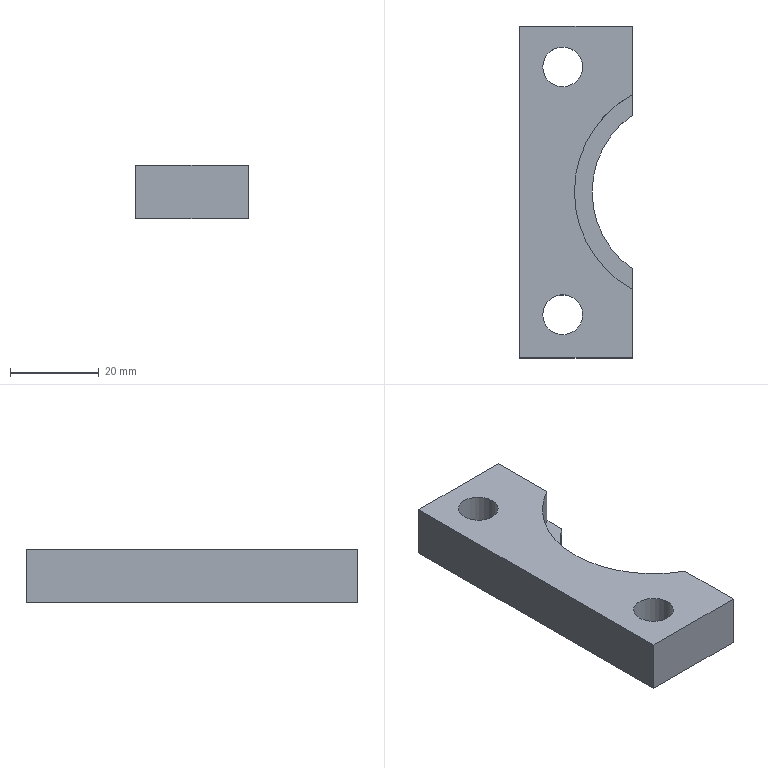Part | NX | features solid 2 | 1 solid | 12 faces | box 25.5 x 75 x 12 mm | volume 17248 mm3 | plane 8 | cylinder 4 | commonest cylinder face diameters 9 x2 42.2 x1 50.2 x1
STEP:
#1=CARTESIAN_POINT('',(697.5,172.5,250.));
#2=VERTEX_POINT('',#1);
#3=CARTESIAN_POINT('',(697.5,247.5,250.));
#4=VERTEX_POINT('',#3);
#5=CARTESIAN_POINT('',(697.5,172.5,250.));
#6=DIRECTION('',(0.,1.,0.));
#7=VECTOR('',#6,1000.);
#8=LINE('',#5,#7);
#9=EDGE_CURVE('',#2,#4,#8,.T.);
#10=ORIENTED_EDGE('',*,*,#9,.T.);
#11=CARTESIAN_POINT('',(697.5,247.5,238.));
#12=VERTEX_POINT('',#11);
#13=CARTESIAN_POINT('',(697.5,247.5,242.));
#14=DIRECTION('',(0.,0.,1.));
#15=VECTOR('',#14,1000.);
#16=LINE('',#13,#15);
#17=EDGE_CURVE('',#12,#4,#16,.T.);
#18=ORIENTED_EDGE('',*,*,#17,.F.);
#19=CARTESIAN_POINT('',(697.5,172.5,238.));
#20=VERTEX_POINT('',#19);
#21=CARTESIAN_POINT('',(697.5,172.5,238.));
#22=DIRECTION('',(0.,1.,0.));
#23=VECTOR('',#22,1000.);
#24=LINE('',#21,#23);
#25=EDGE_CURVE('',#20,#12,#24,.T.);
#26=ORIENTED_EDGE('',*,*,#25,.F.);
#27=CARTESIAN_POINT('',(697.5,172.5,242.));
#28=DIRECTION('',(0.,0.,1.));
#29=VECTOR('',#28,1000.);
#30=LINE('',#27,#29);
#31=EDGE_CURVE('',#20,#2,#30,.T.);
#32=ORIENTED_EDGE('',*,*,#31,.T.);
#33=EDGE_LOOP('',(#10,#18,#26,#32));
#34=FACE_BOUND('',#33,.T.);
#35=CARTESIAN_POINT('',(697.5,172.5,242.));
#36=DIRECTION('',(1.,0.,0.));
#37=DIRECTION('',(0.,0.,-1.));
#38=AXIS2_PLACEMENT_3D('',#35,#36,#37);
#39=PLANE('',#38);
#40=ADVANCED_FACE('',(#34),#39,.F.);
#41=CARTESIAN_POINT('',(723.,172.5,250.));
#42=VERTEX_POINT('',#41);
#43=CARTESIAN_POINT('',(723.,172.5,250.));
#44=DIRECTION('',(-1.,0.,0.));
#45=VECTOR('',#44,1000.);
#46=LINE('',#43,#45);
#47=EDGE_CURVE('',#42,#2,#46,.T.);
#48=ORIENTED_EDGE('',*,*,#47,.T.);
#49=ORIENTED_EDGE('',*,*,#31,.F.);
#50=CARTESIAN_POINT('',(723.,172.5,238.));
#51=VERTEX_POINT('',#50);
#52=CARTESIAN_POINT('',(723.,172.5,238.));
#53=DIRECTION('',(-1.,0.,0.));
#54=VECTOR('',#53,1000.);
#55=LINE('',#52,#54);
#56=EDGE_CURVE('',#51,#20,#55,.T.);
#57=ORIENTED_EDGE('',*,*,#56,.F.);
#58=CARTESIAN_POINT('',(723.,172.5,242.));
#59=DIRECTION('',(0.,0.,1.));
#60=VECTOR('',#59,1000.);
#61=LINE('',#58,#60);
#62=EDGE_CURVE('',#51,#42,#61,.T.);
#63=ORIENTED_EDGE('',*,*,#62,.T.);
#64=EDGE_LOOP('',(#48,#49,#57,#63));
#65=FACE_BOUND('',#64,.T.);
#66=CARTESIAN_POINT('',(723.,172.5,242.));
#67=DIRECTION('',(0.,1.,0.));
#68=DIRECTION('',(0.,0.,1.));
#69=AXIS2_PLACEMENT_3D('',#66,#67,#68);
#70=PLANE('',#69);
#71=ADVANCED_FACE('',(#65),#70,.F.);
#72=CARTESIAN_POINT('',(723.,187.954,250.));
#73=VERTEX_POINT('',#72);
#74=CARTESIAN_POINT('',(723.,192.645,250.));
#75=DIRECTION('',(0.,-1.,0.));
#76=VECTOR('',#75,1000.);
#77=LINE('',#74,#76);
#78=EDGE_CURVE('',#73,#42,#77,.T.);
#79=ORIENTED_EDGE('',*,*,#78,.T.);
#80=ORIENTED_EDGE('',*,*,#62,.F.);
#81=CARTESIAN_POINT('',(723.,192.645,238.));
#82=VERTEX_POINT('',#81);
#83=CARTESIAN_POINT('',(723.,192.645,238.));
#84=DIRECTION('',(0.,-1.,0.));
#85=VECTOR('',#84,1000.);
#86=LINE('',#83,#85);
#87=EDGE_CURVE('',#82,#51,#86,.T.);
#88=ORIENTED_EDGE('',*,*,#87,.F.);
#89=CARTESIAN_POINT('',(723.,192.645,242.));
#90=VERTEX_POINT('',#89);
#91=CARTESIAN_POINT('',(723.,192.645,238.));
#92=DIRECTION('',(0.,0.,1.));
#93=VECTOR('',#92,1000.);
#94=LINE('',#91,#93);
#95=EDGE_CURVE('',#82,#90,#94,.T.);
#96=ORIENTED_EDGE('',*,*,#95,.T.);
#97=CARTESIAN_POINT('',(723.,187.954,242.));
#98=VERTEX_POINT('',#97);
#99=CARTESIAN_POINT('',(723.,192.645,242.));
#100=DIRECTION('',(0.,-1.,0.));
#101=VECTOR('',#100,1000.);
#102=LINE('',#99,#101);
#103=EDGE_CURVE('',#90,#98,#102,.T.);
#104=ORIENTED_EDGE('',*,*,#103,.T.);
#105=CARTESIAN_POINT('',(723.,187.954,242.));
#106=DIRECTION('',(0.,0.,1.));
#107=VECTOR('',#106,1000.);
#108=LINE('',#105,#107);
#109=EDGE_CURVE('',#98,#73,#108,.T.);
#110=ORIENTED_EDGE('',*,*,#109,.T.);
#111=EDGE_LOOP('',(#79,#80,#88,#96,#104,#110));
#112=FACE_BOUND('',#111,.T.);
#113=CARTESIAN_POINT('',(723.,192.645,242.));
#114=DIRECTION('',(-1.,0.,0.));
#115=DIRECTION('',(0.,-1.,0.));
#116=AXIS2_PLACEMENT_3D('',#113,#114,#115);
#117=PLANE('',#116);
#118=ADVANCED_FACE('',(#112),#117,.F.);
#119=CARTESIAN_POINT('',(723.,232.046,250.));
#120=VERTEX_POINT('',#119);
#121=CARTESIAN_POINT('',(735.,210.,250.));
#122=DIRECTION('',(0.,0.,1.));
#123=DIRECTION('',(1.,0.,0.));
#124=AXIS2_PLACEMENT_3D('',#121,#122,#123);
#125=CIRCLE('',#124,25.1);
#126=EDGE_CURVE('',#120,#73,#125,.T.);
#127=ORIENTED_EDGE('',*,*,#126,.T.);
#128=ORIENTED_EDGE('',*,*,#109,.F.);
#129=CARTESIAN_POINT('',(723.,232.046,242.));
#130=VERTEX_POINT('',#129);
#131=CARTESIAN_POINT('',(735.,210.,242.));
#132=DIRECTION('',(0.,0.,1.));
#133=DIRECTION('',(1.,0.,0.));
#134=AXIS2_PLACEMENT_3D('',#131,#132,#133);
#135=CIRCLE('',#134,25.1);
#136=EDGE_CURVE('',#130,#98,#135,.T.);
#137=ORIENTED_EDGE('',*,*,#136,.F.);
#138=CARTESIAN_POINT('',(723.,232.046,242.));
#139=DIRECTION('',(0.,0.,1.));
#140=VECTOR('',#139,1000.);
#141=LINE('',#138,#140);
#142=EDGE_CURVE('',#130,#120,#141,.T.);
#143=ORIENTED_EDGE('',*,*,#142,.T.);
#144=EDGE_LOOP('',(#127,#128,#137,#143));
#145=FACE_BOUND('',#144,.T.);
#146=CARTESIAN_POINT('',(735.,210.,242.));
#147=DIRECTION('',(0.,0.,1.));
#148=DIRECTION('',(1.,0.,0.));
#149=AXIS2_PLACEMENT_3D('',#146,#147,#148);
#150=CYLINDRICAL_SURFACE('',#149,25.1);
#151=ADVANCED_FACE('',(#145),#150,.F.);
#152=CARTESIAN_POINT('',(723.,247.5,250.));
#153=VERTEX_POINT('',#152);
#154=CARTESIAN_POINT('',(723.,247.5,250.));
#155=DIRECTION('',(0.,-1.,0.));
#156=VECTOR('',#155,1000.);
#157=LINE('',#154,#156);
#158=EDGE_CURVE('',#153,#120,#157,.T.);
#159=ORIENTED_EDGE('',*,*,#158,.T.);
#160=ORIENTED_EDGE('',*,*,#142,.F.);
#161=CARTESIAN_POINT('',(723.,227.355,242.));
#162=VERTEX_POINT('',#161);
#163=CARTESIAN_POINT('',(723.,247.5,242.));
#164=DIRECTION('',(0.,-1.,0.));
#165=VECTOR('',#164,1000.);
#166=LINE('',#163,#165);
#167=EDGE_CURVE('',#130,#162,#166,.T.);
#168=ORIENTED_EDGE('',*,*,#167,.T.);
#169=CARTESIAN_POINT('',(723.,227.355,238.));
#170=VERTEX_POINT('',#169);
#171=CARTESIAN_POINT('',(723.,227.355,238.));
#172=DIRECTION('',(0.,0.,1.));
#173=VECTOR('',#172,1000.);
#174=LINE('',#171,#173);
#175=EDGE_CURVE('',#170,#162,#174,.T.);
#176=ORIENTED_EDGE('',*,*,#175,.F.);
#177=CARTESIAN_POINT('',(723.,247.5,238.));
#178=VERTEX_POINT('',#177);
#179=CARTESIAN_POINT('',(723.,247.5,238.));
#180=DIRECTION('',(0.,-1.,0.));
#181=VECTOR('',#180,1000.);
#182=LINE('',#179,#181);
#183=EDGE_CURVE('',#178,#170,#182,.T.);
#184=ORIENTED_EDGE('',*,*,#183,.F.);
#185=CARTESIAN_POINT('',(723.,247.5,242.));
#186=DIRECTION('',(0.,0.,1.));
#187=VECTOR('',#186,1000.);
#188=LINE('',#185,#187);
#189=EDGE_CURVE('',#178,#153,#188,.T.);
#190=ORIENTED_EDGE('',*,*,#189,.T.);
#191=EDGE_LOOP('',(#159,#160,#168,#176,#184,#190));
#192=FACE_BOUND('',#191,.T.);
#193=CARTESIAN_POINT('',(723.,247.5,242.));
#194=DIRECTION('',(-1.,0.,0.));
#195=DIRECTION('',(0.,-1.,0.));
#196=AXIS2_PLACEMENT_3D('',#193,#194,#195);
#197=PLANE('',#196);
#198=ADVANCED_FACE('',(#192),#197,.F.);
#199=CARTESIAN_POINT('',(697.5,247.5,250.));
#200=DIRECTION('',(1.,0.,0.));
#201=VECTOR('',#200,1000.);
#202=LINE('',#199,#201);
#203=EDGE_CURVE('',#4,#153,#202,.T.);
#204=ORIENTED_EDGE('',*,*,#203,.T.);
#205=ORIENTED_EDGE('',*,*,#189,.F.);
#206=CARTESIAN_POINT('',(697.5,247.5,238.));
#207=DIRECTION('',(1.,0.,0.));
#208=VECTOR('',#207,1000.);
#209=LINE('',#206,#208);
#210=EDGE_CURVE('',#12,#178,#209,.T.);
#211=ORIENTED_EDGE('',*,*,#210,.F.);
#212=ORIENTED_EDGE('',*,*,#17,.T.);
#213=EDGE_LOOP('',(#204,#205,#211,#212));
#214=FACE_BOUND('',#213,.T.);
#215=CARTESIAN_POINT('',(697.5,247.5,242.));
#216=DIRECTION('',(0.,-1.,0.));
#217=DIRECTION('',(0.,0.,-1.));
#218=AXIS2_PLACEMENT_3D('',#215,#216,#217);
#219=PLANE('',#218);
#220=ADVANCED_FACE('',(#214),#219,.F.);
#221=CARTESIAN_POINT('',(711.75,238.25,250.));
#222=VERTEX_POINT('',#221);
#223=CARTESIAN_POINT('',(707.25,238.25,250.));
#224=DIRECTION('',(0.,0.,1.));
#225=DIRECTION('',(1.,0.,0.));
#226=AXIS2_PLACEMENT_3D('',#223,#224,#225);
#227=CIRCLE('',#226,4.5);
#228=EDGE_CURVE('',#222,#222,#227,.T.);
#229=ORIENTED_EDGE('',*,*,#228,.F.);
#230=EDGE_LOOP('',(#229));
#231=FACE_BOUND('',#230,.T.);
#232=CARTESIAN_POINT('',(711.75,182.25,250.));
#233=VERTEX_POINT('',#232);
#234=CARTESIAN_POINT('',(707.25,182.25,250.));
#235=DIRECTION('',(0.,0.,1.));
#236=DIRECTION('',(1.,0.,0.));
#237=AXIS2_PLACEMENT_3D('',#234,#235,#236);
#238=CIRCLE('',#237,4.5);
#239=EDGE_CURVE('',#233,#233,#238,.T.);
#240=ORIENTED_EDGE('',*,*,#239,.F.);
#241=EDGE_LOOP('',(#240));
#242=FACE_BOUND('',#241,.T.);
#243=ORIENTED_EDGE('',*,*,#9,.F.);
#244=ORIENTED_EDGE('',*,*,#47,.F.);
#245=ORIENTED_EDGE('',*,*,#78,.F.);
#246=ORIENTED_EDGE('',*,*,#126,.F.);
#247=ORIENTED_EDGE('',*,*,#158,.F.);
#248=ORIENTED_EDGE('',*,*,#203,.F.);
#249=EDGE_LOOP('',(#243,#244,#245,#246,#247,#248));
#250=FACE_BOUND('',#249,.T.);
#251=CARTESIAN_POINT('',(720.683,207.107,250.));
#252=DIRECTION('',(0.,0.,1.));
#253=DIRECTION('',(1.,0.,0.));
#254=AXIS2_PLACEMENT_3D('',#251,#252,#253);
#255=PLANE('',#254);
#256=ADVANCED_FACE('',(#231,#242,#250),#255,.T.);
#257=ORIENTED_EDGE('',*,*,#239,.T.);
#258=EDGE_LOOP('',(#257));
#259=FACE_BOUND('',#258,.T.);
#260=CARTESIAN_POINT('',(711.75,182.25,238.));
#261=VERTEX_POINT('',#260);
#262=CARTESIAN_POINT('',(707.25,182.25,238.));
#263=DIRECTION('',(0.,0.,1.));
#264=DIRECTION('',(1.,0.,0.));
#265=AXIS2_PLACEMENT_3D('',#262,#263,#264);
#266=CIRCLE('',#265,4.5);
#267=EDGE_CURVE('',#261,#261,#266,.T.);
#268=ORIENTED_EDGE('',*,*,#267,.F.);
#269=EDGE_LOOP('',(#268));
#270=FACE_BOUND('',#269,.T.);
#271=CARTESIAN_POINT('',(707.25,182.25,242.));
#272=DIRECTION('',(0.,0.,1.));
#273=DIRECTION('',(1.,0.,0.));
#274=AXIS2_PLACEMENT_3D('',#271,#272,#273);
#275=CYLINDRICAL_SURFACE('',#274,4.5);
#276=ADVANCED_FACE('',(#259,#270),#275,.F.);
#277=ORIENTED_EDGE('',*,*,#228,.T.);
#278=EDGE_LOOP('',(#277));
#279=FACE_BOUND('',#278,.T.);
#280=CARTESIAN_POINT('',(711.75,238.25,238.));
#281=VERTEX_POINT('',#280);
#282=CARTESIAN_POINT('',(707.25,238.25,238.));
#283=DIRECTION('',(0.,0.,1.));
#284=DIRECTION('',(1.,0.,0.));
#285=AXIS2_PLACEMENT_3D('',#282,#283,#284);
#286=CIRCLE('',#285,4.5);
#287=EDGE_CURVE('',#281,#281,#286,.T.);
#288=ORIENTED_EDGE('',*,*,#287,.F.);
#289=EDGE_LOOP('',(#288));
#290=FACE_BOUND('',#289,.T.);
#291=CARTESIAN_POINT('',(707.25,238.25,242.));
#292=DIRECTION('',(0.,0.,1.));
#293=DIRECTION('',(1.,0.,0.));
#294=AXIS2_PLACEMENT_3D('',#291,#292,#293);
#295=CYLINDRICAL_SURFACE('',#294,4.5);
#296=ADVANCED_FACE('',(#279,#290),#295,.F.);
#297=ORIENTED_EDGE('',*,*,#167,.F.);
#298=ORIENTED_EDGE('',*,*,#136,.T.);
#299=ORIENTED_EDGE('',*,*,#103,.F.);
#300=CARTESIAN_POINT('',(735.,210.,242.));
#301=DIRECTION('',(0.,0.,1.));
#302=DIRECTION('',(1.,0.,0.));
#303=AXIS2_PLACEMENT_3D('',#300,#301,#302);
#304=CIRCLE('',#303,21.1);
#305=EDGE_CURVE('',#162,#90,#304,.T.);
#306=ORIENTED_EDGE('',*,*,#305,.F.);
#307=EDGE_LOOP('',(#297,#298,#299,#306));
#308=FACE_BOUND('',#307,.T.);
#309=CARTESIAN_POINT('',(735.,210.,242.));
#310=DIRECTION('',(0.,0.,1.));
#311=DIRECTION('',(1.,0.,0.));
#312=AXIS2_PLACEMENT_3D('',#309,#310,#311);
#313=PLANE('',#312);
#314=ADVANCED_FACE('',(#308),#313,.T.);
#315=ORIENTED_EDGE('',*,*,#287,.T.);
#316=EDGE_LOOP('',(#315));
#317=FACE_BOUND('',#316,.T.);
#318=ORIENTED_EDGE('',*,*,#267,.T.);
#319=EDGE_LOOP('',(#318));
#320=FACE_BOUND('',#319,.T.);
#321=ORIENTED_EDGE('',*,*,#87,.T.);
#322=ORIENTED_EDGE('',*,*,#56,.T.);
#323=ORIENTED_EDGE('',*,*,#25,.T.);
#324=ORIENTED_EDGE('',*,*,#210,.T.);
#325=ORIENTED_EDGE('',*,*,#183,.T.);
#326=CARTESIAN_POINT('',(735.,210.,238.));
#327=DIRECTION('',(0.,0.,1.));
#328=DIRECTION('',(1.,0.,0.));
#329=AXIS2_PLACEMENT_3D('',#326,#327,#328);
#330=CIRCLE('',#329,21.1);
#331=EDGE_CURVE('',#170,#82,#330,.T.);
#332=ORIENTED_EDGE('',*,*,#331,.T.);
#333=EDGE_LOOP('',(#321,#322,#323,#324,#325,#332));
#334=FACE_BOUND('',#333,.T.);
#335=CARTESIAN_POINT('',(735.,210.,238.));
#336=DIRECTION('',(0.,0.,1.));
#337=DIRECTION('',(1.,0.,0.));
#338=AXIS2_PLACEMENT_3D('',#335,#336,#337);
#339=PLANE('',#338);
#340=ADVANCED_FACE('',(#317,#320,#334),#339,.F.);
#341=ORIENTED_EDGE('',*,*,#305,.T.);
#342=ORIENTED_EDGE('',*,*,#95,.F.);
#343=ORIENTED_EDGE('',*,*,#331,.F.);
#344=ORIENTED_EDGE('',*,*,#175,.T.);
#345=EDGE_LOOP('',(#341,#342,#343,#344));
#346=FACE_BOUND('',#345,.T.);
#347=CARTESIAN_POINT('',(735.,210.,238.));
#348=DIRECTION('',(0.,0.,1.));
#349=DIRECTION('',(1.,0.,0.));
#350=AXIS2_PLACEMENT_3D('',#347,#348,#349);
#351=CYLINDRICAL_SURFACE('',#350,21.1);
#352=ADVANCED_FACE('',(#346),#351,.F.);
#353=CLOSED_SHELL('',(#40,#71,#118,#151,#198,#220,#256,#276,#296,#314,#340,#352));
#354=MANIFOLD_SOLID_BREP('',#353);
#355=(LENGTH_UNIT()NAMED_UNIT(*)SI_UNIT(.MILLI.,.METRE.));
#356=UNCERTAINTY_MEASURE_WITH_UNIT(LENGTH_MEASURE(0.00001),#355,'','');
#357=(NAMED_UNIT(*)PLANE_ANGLE_UNIT()SI_UNIT($,.RADIAN.));
#358=(NAMED_UNIT(*)SI_UNIT($,.STERADIAN.)SOLID_ANGLE_UNIT());
#359=(GEOMETRIC_REPRESENTATION_CONTEXT(3)GLOBAL_UNCERTAINTY_ASSIGNED_CONTEXT((#356))GLOBAL_UNIT_ASSIGNED_CONTEXT((#355,#357,#358))REPRESENTATION_CONTEXT('',''));
#360=ADVANCED_BREP_SHAPE_REPRESENTATION('',(#354),#359);